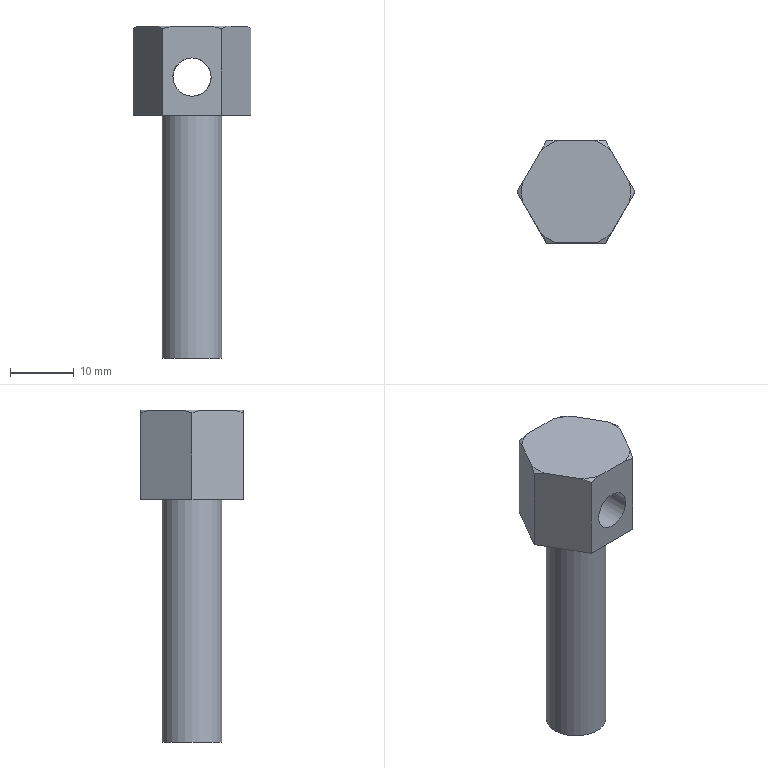Part | NX | features DATUM_CSYS 3, EXTRUDE 3, SKETCH 2, CHAMFER 1, CYLINDER 1, HOLE PACKAGE 1, SIMPLE HOLE 1, SYMBOLIC_THREAD 1 | 1 solid | 18 faces | box 18.475 x 16 x 52 mm | volume 4103 mm3 | plane 9 | cone 6 | cylinder 3 | commonest cylinder face diameters 6 x2 9.373 x1
STEP:
#1=CARTESIAN_POINT('',(4.619,8.,13.587));
#2=VERTEX_POINT('',#1);
#3=CARTESIAN_POINT('',(2.94,8.,14.));
#4=VERTEX_POINT('',#3);
#5=CARTESIAN_POINT('',(4.619,8.,13.587));
#6=CARTESIAN_POINT('',(4.067,8.,13.747));
#7=CARTESIAN_POINT('',(3.508,8.,13.887));
#8=CARTESIAN_POINT('',(2.94,8.,14.));
#9=B_SPLINE_CURVE_WITH_KNOTS('',3,(#5,#6,#7,#8),.UNSPECIFIED.,.F.,.F.,(4,4),(0.005943,0.007663),.UNSPECIFIED.);
#10=EDGE_CURVE('',#2,#4,#9,.T.);
#11=ORIENTED_EDGE('',*,*,#10,.F.);
#12=CARTESIAN_POINT('',(4.619,8.,0.));
#13=VERTEX_POINT('',#12);
#14=CARTESIAN_POINT('',(4.619,8.,14.));
#15=DIRECTION('',(0.,0.,-1.));
#16=VECTOR('',#15,1000.);
#17=LINE('',#14,#16);
#18=EDGE_CURVE('',#2,#13,#17,.T.);
#19=ORIENTED_EDGE('',*,*,#18,.T.);
#20=CARTESIAN_POINT('',(-4.619,8.,0.));
#21=VERTEX_POINT('',#20);
#22=CARTESIAN_POINT('',(-4.619,8.,0.));
#23=DIRECTION('',(1.,0.,0.));
#24=VECTOR('',#23,1000.);
#25=LINE('',#22,#24);
#26=EDGE_CURVE('',#21,#13,#25,.T.);
#27=ORIENTED_EDGE('',*,*,#26,.F.);
#28=CARTESIAN_POINT('',(-4.619,8.,13.587));
#29=VERTEX_POINT('',#28);
#30=CARTESIAN_POINT('',(-4.619,8.,14.));
#31=DIRECTION('',(0.,0.,-1.));
#32=VECTOR('',#31,1000.);
#33=LINE('',#30,#32);
#34=EDGE_CURVE('',#29,#21,#33,.T.);
#35=ORIENTED_EDGE('',*,*,#34,.F.);
#36=CARTESIAN_POINT('',(-2.94,8.,14.));
#37=VERTEX_POINT('',#36);
#38=CARTESIAN_POINT('',(-2.94,8.,14.));
#39=CARTESIAN_POINT('',(-3.508,8.,13.887));
#40=CARTESIAN_POINT('',(-4.067,8.,13.747));
#41=CARTESIAN_POINT('',(-4.619,8.,13.587));
#42=B_SPLINE_CURVE_WITH_KNOTS('',3,(#38,#39,#40,#41),.UNSPECIFIED.,.F.,.F.,(4,4),(0.01358,0.01531),.UNSPECIFIED.);
#43=EDGE_CURVE('',#37,#29,#42,.T.);
#44=ORIENTED_EDGE('',*,*,#43,.F.);
#45=CARTESIAN_POINT('',(-4.619,8.,14.));
#46=DIRECTION('',(1.,0.,0.));
#47=VECTOR('',#46,1000.);
#48=LINE('',#45,#47);
#49=EDGE_CURVE('',#37,#4,#48,.T.);
#50=ORIENTED_EDGE('',*,*,#49,.T.);
#51=EDGE_LOOP('',(#11,#19,#27,#35,#44,#50));
#52=FACE_BOUND('',#51,.T.);
#53=CARTESIAN_POINT('',(0.,8.,9.));
#54=VERTEX_POINT('',#53);
#55=CARTESIAN_POINT('',(0.,8.,6.));
#56=DIRECTION('',(0.,1.,0.));
#57=DIRECTION('',(0.,0.,1.));
#58=AXIS2_PLACEMENT_3D('',#55,#56,#57);
#59=CIRCLE('',#58,3.);
#60=EDGE_CURVE('',#54,#54,#59,.F.);
#61=ORIENTED_EDGE('',*,*,#60,.T.);
#62=EDGE_LOOP('',(#61));
#63=FACE_BOUND('',#62,.T.);
#64=CARTESIAN_POINT('',(-4.619,8.,14.));
#65=DIRECTION('',(0.,1.,0.));
#66=DIRECTION('',(0.,0.,1.));
#67=AXIS2_PLACEMENT_3D('',#64,#65,#66);
#68=PLANE('',#67);
#69=ADVANCED_FACE('',(#52,#63),#68,.T.);
#70=CARTESIAN_POINT('',(-4.619,-8.,13.587));
#71=VERTEX_POINT('',#70);
#72=CARTESIAN_POINT('',(-2.94,-8.,14.));
#73=VERTEX_POINT('',#72);
#74=CARTESIAN_POINT('',(-4.619,-8.,13.587));
#75=CARTESIAN_POINT('',(-4.067,-8.,13.747));
#76=CARTESIAN_POINT('',(-3.508,-8.,13.887));
#77=CARTESIAN_POINT('',(-2.94,-8.,14.));
#78=B_SPLINE_CURVE_WITH_KNOTS('',3,(#74,#75,#76,#77),.UNSPECIFIED.,.F.,.F.,(4,4),(0.005943,0.007663),.UNSPECIFIED.);
#79=EDGE_CURVE('',#71,#73,#78,.T.);
#80=ORIENTED_EDGE('',*,*,#79,.F.);
#81=CARTESIAN_POINT('',(-4.619,-8.,0.));
#82=VERTEX_POINT('',#81);
#83=CARTESIAN_POINT('',(-4.619,-8.,14.));
#84=DIRECTION('',(0.,0.,-1.));
#85=VECTOR('',#84,1000.);
#86=LINE('',#83,#85);
#87=EDGE_CURVE('',#71,#82,#86,.T.);
#88=ORIENTED_EDGE('',*,*,#87,.T.);
#89=CARTESIAN_POINT('',(4.619,-8.,0.));
#90=VERTEX_POINT('',#89);
#91=CARTESIAN_POINT('',(4.619,-8.,0.));
#92=DIRECTION('',(-1.,0.,0.));
#93=VECTOR('',#92,1000.);
#94=LINE('',#91,#93);
#95=EDGE_CURVE('',#90,#82,#94,.T.);
#96=ORIENTED_EDGE('',*,*,#95,.F.);
#97=CARTESIAN_POINT('',(4.619,-8.,13.587));
#98=VERTEX_POINT('',#97);
#99=CARTESIAN_POINT('',(4.619,-8.,14.));
#100=DIRECTION('',(0.,0.,-1.));
#101=VECTOR('',#100,1000.);
#102=LINE('',#99,#101);
#103=EDGE_CURVE('',#98,#90,#102,.T.);
#104=ORIENTED_EDGE('',*,*,#103,.F.);
#105=CARTESIAN_POINT('',(2.94,-8.,14.));
#106=VERTEX_POINT('',#105);
#107=CARTESIAN_POINT('',(2.94,-8.,14.));
#108=CARTESIAN_POINT('',(3.508,-8.,13.887));
#109=CARTESIAN_POINT('',(4.067,-8.,13.747));
#110=CARTESIAN_POINT('',(4.619,-8.,13.587));
#111=B_SPLINE_CURVE_WITH_KNOTS('',3,(#107,#108,#109,#110),.UNSPECIFIED.,.F.,.F.,(4,4),(0.01358,0.01531),.UNSPECIFIED.);
#112=EDGE_CURVE('',#106,#98,#111,.T.);
#113=ORIENTED_EDGE('',*,*,#112,.F.);
#114=CARTESIAN_POINT('',(4.619,-8.,14.));
#115=DIRECTION('',(-1.,0.,0.));
#116=VECTOR('',#115,1000.);
#117=LINE('',#114,#116);
#118=EDGE_CURVE('',#106,#73,#117,.T.);
#119=ORIENTED_EDGE('',*,*,#118,.T.);
#120=EDGE_LOOP('',(#80,#88,#96,#104,#113,#119));
#121=FACE_BOUND('',#120,.T.);
#122=CARTESIAN_POINT('',(3.,-8.,6.));
#123=VERTEX_POINT('',#122);
#124=CARTESIAN_POINT('',(0.,-8.,6.));
#125=DIRECTION('',(0.,-1.,0.));
#126=DIRECTION('',(1.,0.,0.));
#127=AXIS2_PLACEMENT_3D('',#124,#125,#126);
#128=CIRCLE('',#127,3.);
#129=EDGE_CURVE('',#123,#123,#128,.F.);
#130=ORIENTED_EDGE('',*,*,#129,.T.);
#131=EDGE_LOOP('',(#130));
#132=FACE_BOUND('',#131,.T.);
#133=CARTESIAN_POINT('',(4.619,-8.,14.));
#134=DIRECTION('',(0.,-1.,0.));
#135=DIRECTION('',(1.,0.,0.));
#136=AXIS2_PLACEMENT_3D('',#133,#134,#135);
#137=PLANE('',#136);
#138=ADVANCED_FACE('',(#121,#132),#137,.T.);
#139=CARTESIAN_POINT('',(3.,0.,-38.));
#140=VERTEX_POINT('',#139);
#141=CARTESIAN_POINT('',(0.,0.,-38.));
#142=DIRECTION('',(0.,0.,1.));
#143=DIRECTION('',(1.,0.,0.));
#144=AXIS2_PLACEMENT_3D('',#141,#142,#143);
#145=CIRCLE('',#144,3.);
#146=EDGE_CURVE('',#140,#140,#145,.T.);
#147=ORIENTED_EDGE('',*,*,#146,.F.);
#148=EDGE_LOOP('',(#147));
#149=FACE_BOUND('',#148,.T.);
#150=CARTESIAN_POINT('',(-3.,0.,6.));
#151=VERTEX_POINT('',#150);
#152=CARTESIAN_POINT('',(3.,0.,6.));
#153=VERTEX_POINT('',#152);
#154=CARTESIAN_POINT('',(0.,0.,6.));
#155=DIRECTION('',(0.,0.7071,0.7071));
#156=DIRECTION('',(0.,-0.7071,0.7071));
#157=AXIS2_PLACEMENT_3D('',#154,#155,#156);
#158=ELLIPSE('',#157,4.243,3.);
#159=EDGE_CURVE('',#151,#153,#158,.F.);
#160=ORIENTED_EDGE('',*,*,#159,.F.);
#161=CARTESIAN_POINT('',(0.,0.,6.));
#162=DIRECTION('',(0.,-0.7071,0.7071));
#163=DIRECTION('',(0.,0.7071,0.7071));
#164=AXIS2_PLACEMENT_3D('',#161,#162,#163);
#165=ELLIPSE('',#164,4.243,3.);
#166=EDGE_CURVE('',#153,#151,#165,.F.);
#167=ORIENTED_EDGE('',*,*,#166,.F.);
#168=EDGE_LOOP('',(#160,#167));
#169=FACE_BOUND('',#168,.T.);
#170=CARTESIAN_POINT('',(0.,0.,-38.));
#171=DIRECTION('',(0.,0.,1.));
#172=DIRECTION('',(1.,0.,0.));
#173=AXIS2_PLACEMENT_3D('',#170,#171,#172);
#174=CYLINDRICAL_SURFACE('',#173,3.);
#175=ADVANCED_FACE('',(#149,#169),#174,.F.);
#176=CARTESIAN_POINT('',(-8.398,1.454,14.));
#177=VERTEX_POINT('',#176);
#178=CARTESIAN_POINT('',(-9.238,0.,13.587));
#179=VERTEX_POINT('',#178);
#180=CARTESIAN_POINT('',(-8.398,1.454,14.));
#181=CARTESIAN_POINT('',(-8.682,0.963,13.887));
#182=CARTESIAN_POINT('',(-8.961,0.4789,13.747));
#183=CARTESIAN_POINT('',(-9.238,0.,13.587));
#184=B_SPLINE_CURVE_WITH_KNOTS('',3,(#180,#181,#182,#183),.UNSPECIFIED.,.F.,.F.,(4,4),(0.01453,0.01627),.UNSPECIFIED.);
#185=EDGE_CURVE('',#177,#179,#184,.T.);
#186=ORIENTED_EDGE('',*,*,#185,.T.);
#187=CARTESIAN_POINT('',(-8.398,-1.454,14.));
#188=VERTEX_POINT('',#187);
#189=CARTESIAN_POINT('',(-9.238,0.,13.587));
#190=CARTESIAN_POINT('',(-8.961,-0.479,13.747));
#191=CARTESIAN_POINT('',(-8.68,-0.9662,13.888));
#192=CARTESIAN_POINT('',(-8.398,-1.454,14.));
#193=B_SPLINE_CURVE_WITH_KNOTS('',3,(#189,#190,#191,#192),.UNSPECIFIED.,.F.,.F.,(4,4),(0.006888,0.008609),.UNSPECIFIED.);
#194=EDGE_CURVE('',#179,#188,#193,.T.);
#195=ORIENTED_EDGE('',*,*,#194,.T.);
#196=CARTESIAN_POINT('',(0.,0.,14.));
#197=DIRECTION('',(0.,0.,1.));
#198=DIRECTION('',(1.,0.,0.));
#199=AXIS2_PLACEMENT_3D('',#196,#197,#198);
#200=CIRCLE('',#199,8.523);
#201=EDGE_CURVE('',#177,#188,#200,.T.);
#202=ORIENTED_EDGE('',*,*,#201,.F.);
#203=EDGE_LOOP('',(#186,#195,#202));
#204=FACE_BOUND('',#203,.T.);
#205=CARTESIAN_POINT('',(0.,0.,14.));
#206=DIRECTION('',(0.,0.,-1.));
#207=DIRECTION('',(-1.,0.,0.));
#208=AXIS2_PLACEMENT_3D('',#205,#206,#207);
#209=CONICAL_SURFACE('',#208,8.523,1.047);
#210=ADVANCED_FACE('',(#204),#209,.T.);
#211=ORIENTED_EDGE('',*,*,#43,.T.);
#212=CARTESIAN_POINT('',(-5.458,6.546,14.));
#213=VERTEX_POINT('',#212);
#214=CARTESIAN_POINT('',(-4.619,8.,13.587));
#215=CARTESIAN_POINT('',(-4.895,7.521,13.747));
#216=CARTESIAN_POINT('',(-5.177,7.034,13.888));
#217=CARTESIAN_POINT('',(-5.458,6.546,14.));
#218=B_SPLINE_CURVE_WITH_KNOTS('',3,(#214,#215,#216,#217),.UNSPECIFIED.,.F.,.F.,(4,4),(0.006888,0.008609),.UNSPECIFIED.);
#219=EDGE_CURVE('',#29,#213,#218,.T.);
#220=ORIENTED_EDGE('',*,*,#219,.T.);
#221=CARTESIAN_POINT('',(0.,0.,14.));
#222=DIRECTION('',(0.,0.,1.));
#223=DIRECTION('',(1.,0.,0.));
#224=AXIS2_PLACEMENT_3D('',#221,#222,#223);
#225=CIRCLE('',#224,8.523);
#226=EDGE_CURVE('',#37,#213,#225,.T.);
#227=ORIENTED_EDGE('',*,*,#226,.F.);
#228=EDGE_LOOP('',(#211,#220,#227));
#229=FACE_BOUND('',#228,.T.);
#230=CARTESIAN_POINT('',(0.,0.,14.));
#231=DIRECTION('',(0.,0.,-1.));
#232=DIRECTION('',(-1.,0.,0.));
#233=AXIS2_PLACEMENT_3D('',#230,#231,#232);
#234=CONICAL_SURFACE('',#233,8.523,1.047);
#235=ADVANCED_FACE('',(#229),#234,.T.);
#236=CARTESIAN_POINT('',(5.458,6.546,14.));
#237=VERTEX_POINT('',#236);
#238=CARTESIAN_POINT('',(5.458,6.546,14.));
#239=CARTESIAN_POINT('',(5.175,7.037,13.887));
#240=CARTESIAN_POINT('',(4.895,7.521,13.747));
#241=CARTESIAN_POINT('',(4.619,8.,13.587));
#242=B_SPLINE_CURVE_WITH_KNOTS('',3,(#238,#239,#240,#241),.UNSPECIFIED.,.F.,.F.,(4,4),(0.01453,0.01627),.UNSPECIFIED.);
#243=EDGE_CURVE('',#237,#2,#242,.T.);
#244=ORIENTED_EDGE('',*,*,#243,.T.);
#245=ORIENTED_EDGE('',*,*,#10,.T.);
#246=CARTESIAN_POINT('',(0.,0.,14.));
#247=DIRECTION('',(0.,0.,1.));
#248=DIRECTION('',(1.,0.,0.));
#249=AXIS2_PLACEMENT_3D('',#246,#247,#248);
#250=CIRCLE('',#249,8.523);
#251=EDGE_CURVE('',#237,#4,#250,.T.);
#252=ORIENTED_EDGE('',*,*,#251,.F.);
#253=EDGE_LOOP('',(#244,#245,#252));
#254=FACE_BOUND('',#253,.T.);
#255=CARTESIAN_POINT('',(0.,0.,14.));
#256=DIRECTION('',(0.,0.,-1.));
#257=DIRECTION('',(-1.,0.,0.));
#258=AXIS2_PLACEMENT_3D('',#255,#256,#257);
#259=CONICAL_SURFACE('',#258,8.523,1.047);
#260=ADVANCED_FACE('',(#254),#259,.T.);
#261=CARTESIAN_POINT('',(8.398,-1.454,14.));
#262=VERTEX_POINT('',#261);
#263=CARTESIAN_POINT('',(9.238,0.,13.587));
#264=VERTEX_POINT('',#263);
#265=CARTESIAN_POINT('',(8.398,-1.454,14.));
#266=CARTESIAN_POINT('',(8.682,-0.963,13.887));
#267=CARTESIAN_POINT('',(8.961,-0.4789,13.747));
#268=CARTESIAN_POINT('',(9.238,0.,13.587));
#269=B_SPLINE_CURVE_WITH_KNOTS('',3,(#265,#266,#267,#268),.UNSPECIFIED.,.F.,.F.,(4,4),(0.01453,0.01627),.UNSPECIFIED.);
#270=EDGE_CURVE('',#262,#264,#269,.T.);
#271=ORIENTED_EDGE('',*,*,#270,.T.);
#272=CARTESIAN_POINT('',(8.398,1.454,14.));
#273=VERTEX_POINT('',#272);
#274=CARTESIAN_POINT('',(9.238,0.,13.587));
#275=CARTESIAN_POINT('',(8.961,0.479,13.747));
#276=CARTESIAN_POINT('',(8.68,0.9662,13.888));
#277=CARTESIAN_POINT('',(8.398,1.454,14.));
#278=B_SPLINE_CURVE_WITH_KNOTS('',3,(#274,#275,#276,#277),.UNSPECIFIED.,.F.,.F.,(4,4),(0.006888,0.008609),.UNSPECIFIED.);
#279=EDGE_CURVE('',#264,#273,#278,.T.);
#280=ORIENTED_EDGE('',*,*,#279,.T.);
#281=CARTESIAN_POINT('',(0.,0.,14.));
#282=DIRECTION('',(0.,0.,1.));
#283=DIRECTION('',(1.,0.,0.));
#284=AXIS2_PLACEMENT_3D('',#281,#282,#283);
#285=CIRCLE('',#284,8.523);
#286=EDGE_CURVE('',#262,#273,#285,.T.);
#287=ORIENTED_EDGE('',*,*,#286,.F.);
#288=EDGE_LOOP('',(#271,#280,#287));
#289=FACE_BOUND('',#288,.T.);
#290=CARTESIAN_POINT('',(0.,0.,14.));
#291=DIRECTION('',(0.,0.,-1.));
#292=DIRECTION('',(-1.,0.,0.));
#293=AXIS2_PLACEMENT_3D('',#290,#291,#292);
#294=CONICAL_SURFACE('',#293,8.523,1.047);
#295=ADVANCED_FACE('',(#289),#294,.T.);
#296=ORIENTED_EDGE('',*,*,#112,.T.);
#297=CARTESIAN_POINT('',(5.458,-6.546,14.));
#298=VERTEX_POINT('',#297);
#299=CARTESIAN_POINT('',(4.619,-8.,13.587));
#300=CARTESIAN_POINT('',(4.895,-7.521,13.747));
#301=CARTESIAN_POINT('',(5.177,-7.034,13.888));
#302=CARTESIAN_POINT('',(5.458,-6.546,14.));
#303=B_SPLINE_CURVE_WITH_KNOTS('',3,(#299,#300,#301,#302),.UNSPECIFIED.,.F.,.F.,(4,4),(0.006888,0.008609),.UNSPECIFIED.);
#304=EDGE_CURVE('',#98,#298,#303,.T.);
#305=ORIENTED_EDGE('',*,*,#304,.T.);
#306=CARTESIAN_POINT('',(0.,0.,14.));
#307=DIRECTION('',(0.,0.,1.));
#308=DIRECTION('',(1.,0.,0.));
#309=AXIS2_PLACEMENT_3D('',#306,#307,#308);
#310=CIRCLE('',#309,8.523);
#311=EDGE_CURVE('',#106,#298,#310,.T.);
#312=ORIENTED_EDGE('',*,*,#311,.F.);
#313=EDGE_LOOP('',(#296,#305,#312));
#314=FACE_BOUND('',#313,.T.);
#315=CARTESIAN_POINT('',(0.,0.,14.));
#316=DIRECTION('',(0.,0.,-1.));
#317=DIRECTION('',(-1.,0.,0.));
#318=AXIS2_PLACEMENT_3D('',#315,#316,#317);
#319=CONICAL_SURFACE('',#318,8.523,1.047);
#320=ADVANCED_FACE('',(#314),#319,.T.);
#321=CARTESIAN_POINT('',(-5.458,-6.546,14.));
#322=VERTEX_POINT('',#321);
#323=CARTESIAN_POINT('',(0.,0.,14.));
#324=DIRECTION('',(0.,0.,1.));
#325=DIRECTION('',(1.,0.,0.));
#326=AXIS2_PLACEMENT_3D('',#323,#324,#325);
#327=CIRCLE('',#326,8.523);
#328=EDGE_CURVE('',#322,#73,#327,.T.);
#329=ORIENTED_EDGE('',*,*,#328,.F.);
#330=CARTESIAN_POINT('',(-5.458,-6.546,14.));
#331=CARTESIAN_POINT('',(-5.175,-7.037,13.887));
#332=CARTESIAN_POINT('',(-4.895,-7.521,13.747));
#333=CARTESIAN_POINT('',(-4.619,-8.,13.587));
#334=B_SPLINE_CURVE_WITH_KNOTS('',3,(#330,#331,#332,#333),.UNSPECIFIED.,.F.,.F.,(4,4),(0.01453,0.01627),.UNSPECIFIED.);
#335=EDGE_CURVE('',#322,#71,#334,.T.);
#336=ORIENTED_EDGE('',*,*,#335,.T.);
#337=ORIENTED_EDGE('',*,*,#79,.T.);
#338=EDGE_LOOP('',(#329,#336,#337));
#339=FACE_BOUND('',#338,.T.);
#340=CARTESIAN_POINT('',(0.,0.,14.));
#341=DIRECTION('',(0.,0.,-1.));
#342=DIRECTION('',(-1.,0.,0.));
#343=AXIS2_PLACEMENT_3D('',#340,#341,#342);
#344=CONICAL_SURFACE('',#343,8.523,1.047);
#345=ADVANCED_FACE('',(#339),#344,.T.);
#346=CARTESIAN_POINT('',(-4.619,-8.,14.));
#347=DIRECTION('',(-0.5,0.866,0.));
#348=VECTOR('',#347,1000.);
#349=LINE('',#346,#348);
#350=EDGE_CURVE('',#322,#188,#349,.T.);
#351=ORIENTED_EDGE('',*,*,#350,.F.);
#352=ORIENTED_EDGE('',*,*,#328,.T.);
#353=ORIENTED_EDGE('',*,*,#118,.F.);
#354=ORIENTED_EDGE('',*,*,#311,.T.);
#355=CARTESIAN_POINT('',(9.238,0.,14.));
#356=DIRECTION('',(-0.5,-0.866,0.));
#357=VECTOR('',#356,1000.);
#358=LINE('',#355,#357);
#359=EDGE_CURVE('',#262,#298,#358,.T.);
#360=ORIENTED_EDGE('',*,*,#359,.F.);
#361=ORIENTED_EDGE('',*,*,#286,.T.);
#362=CARTESIAN_POINT('',(4.619,8.,14.));
#363=DIRECTION('',(0.5,-0.866,0.));
#364=VECTOR('',#363,1000.);
#365=LINE('',#362,#364);
#366=EDGE_CURVE('',#237,#273,#365,.T.);
#367=ORIENTED_EDGE('',*,*,#366,.F.);
#368=ORIENTED_EDGE('',*,*,#251,.T.);
#369=ORIENTED_EDGE('',*,*,#49,.F.);
#370=ORIENTED_EDGE('',*,*,#226,.T.);
#371=CARTESIAN_POINT('',(-9.238,0.,14.));
#372=DIRECTION('',(0.5,0.866,0.));
#373=VECTOR('',#372,1000.);
#374=LINE('',#371,#373);
#375=EDGE_CURVE('',#177,#213,#374,.T.);
#376=ORIENTED_EDGE('',*,*,#375,.F.);
#377=ORIENTED_EDGE('',*,*,#201,.T.);
#378=EDGE_LOOP('',(#351,#352,#353,#354,#360,#361,#367,#368,#369,#370,#376,#377));
#379=FACE_BOUND('',#378,.T.);
#380=CARTESIAN_POINT('',(0.,0.,14.));
#381=DIRECTION('',(0.,0.,1.));
#382=DIRECTION('',(1.,0.,0.));
#383=AXIS2_PLACEMENT_3D('',#380,#381,#382);
#384=PLANE('',#383);
#385=ADVANCED_FACE('',(#379),#384,.T.);
#386=ORIENTED_EDGE('',*,*,#194,.F.);
#387=CARTESIAN_POINT('',(-9.238,0.,0.));
#388=VERTEX_POINT('',#387);
#389=CARTESIAN_POINT('',(-9.238,0.,14.));
#390=DIRECTION('',(0.,0.,-1.));
#391=VECTOR('',#390,1000.);
#392=LINE('',#389,#391);
#393=EDGE_CURVE('',#179,#388,#392,.T.);
#394=ORIENTED_EDGE('',*,*,#393,.T.);
#395=CARTESIAN_POINT('',(-4.619,-8.,0.));
#396=DIRECTION('',(-0.5,0.866,0.));
#397=VECTOR('',#396,1000.);
#398=LINE('',#395,#397);
#399=EDGE_CURVE('',#82,#388,#398,.T.);
#400=ORIENTED_EDGE('',*,*,#399,.F.);
#401=ORIENTED_EDGE('',*,*,#87,.F.);
#402=ORIENTED_EDGE('',*,*,#335,.F.);
#403=ORIENTED_EDGE('',*,*,#350,.T.);
#404=EDGE_LOOP('',(#386,#394,#400,#401,#402,#403));
#405=FACE_BOUND('',#404,.T.);
#406=CARTESIAN_POINT('',(-4.619,-8.,14.));
#407=DIRECTION('',(-0.866,-0.5,0.));
#408=DIRECTION('',(0.5,-0.866,0.));
#409=AXIS2_PLACEMENT_3D('',#406,#407,#408);
#410=PLANE('',#409);
#411=ADVANCED_FACE('',(#405),#410,.T.);
#412=ORIENTED_EDGE('',*,*,#219,.F.);
#413=ORIENTED_EDGE('',*,*,#34,.T.);
#414=CARTESIAN_POINT('',(-9.238,0.,0.));
#415=DIRECTION('',(0.5,0.866,0.));
#416=VECTOR('',#415,1000.);
#417=LINE('',#414,#416);
#418=EDGE_CURVE('',#388,#21,#417,.T.);
#419=ORIENTED_EDGE('',*,*,#418,.F.);
#420=ORIENTED_EDGE('',*,*,#393,.F.);
#421=ORIENTED_EDGE('',*,*,#185,.F.);
#422=ORIENTED_EDGE('',*,*,#375,.T.);
#423=EDGE_LOOP('',(#412,#413,#419,#420,#421,#422));
#424=FACE_BOUND('',#423,.T.);
#425=CARTESIAN_POINT('',(-9.238,0.,14.));
#426=DIRECTION('',(-0.866,0.5,0.));
#427=DIRECTION('',(-0.5,-0.866,0.));
#428=AXIS2_PLACEMENT_3D('',#425,#426,#427);
#429=PLANE('',#428);
#430=ADVANCED_FACE('',(#424),#429,.T.);
#431=ORIENTED_EDGE('',*,*,#279,.F.);
#432=CARTESIAN_POINT('',(9.238,0.,0.));
#433=VERTEX_POINT('',#432);
#434=CARTESIAN_POINT('',(9.238,0.,14.));
#435=DIRECTION('',(0.,0.,-1.));
#436=VECTOR('',#435,1000.);
#437=LINE('',#434,#436);
#438=EDGE_CURVE('',#264,#433,#437,.T.);
#439=ORIENTED_EDGE('',*,*,#438,.T.);
#440=CARTESIAN_POINT('',(4.619,8.,0.));
#441=DIRECTION('',(0.5,-0.866,0.));
#442=VECTOR('',#441,1000.);
#443=LINE('',#440,#442);
#444=EDGE_CURVE('',#13,#433,#443,.T.);
#445=ORIENTED_EDGE('',*,*,#444,.F.);
#446=ORIENTED_EDGE('',*,*,#18,.F.);
#447=ORIENTED_EDGE('',*,*,#243,.F.);
#448=ORIENTED_EDGE('',*,*,#366,.T.);
#449=EDGE_LOOP('',(#431,#439,#445,#446,#447,#448));
#450=FACE_BOUND('',#449,.T.);
#451=CARTESIAN_POINT('',(4.619,8.,14.));
#452=DIRECTION('',(0.866,0.5,0.));
#453=DIRECTION('',(-0.5,0.866,0.));
#454=AXIS2_PLACEMENT_3D('',#451,#452,#453);
#455=PLANE('',#454);
#456=ADVANCED_FACE('',(#450),#455,.T.);
#457=ORIENTED_EDGE('',*,*,#304,.F.);
#458=ORIENTED_EDGE('',*,*,#103,.T.);
#459=CARTESIAN_POINT('',(9.238,0.,0.));
#460=DIRECTION('',(-0.5,-0.866,0.));
#461=VECTOR('',#460,1000.);
#462=LINE('',#459,#461);
#463=EDGE_CURVE('',#433,#90,#462,.T.);
#464=ORIENTED_EDGE('',*,*,#463,.F.);
#465=ORIENTED_EDGE('',*,*,#438,.F.);
#466=ORIENTED_EDGE('',*,*,#270,.F.);
#467=ORIENTED_EDGE('',*,*,#359,.T.);
#468=EDGE_LOOP('',(#457,#458,#464,#465,#466,#467));
#469=FACE_BOUND('',#468,.T.);
#470=CARTESIAN_POINT('',(9.238,0.,14.));
#471=DIRECTION('',(0.866,-0.5,0.));
#472=DIRECTION('',(0.5,0.866,0.));
#473=AXIS2_PLACEMENT_3D('',#470,#471,#472);
#474=PLANE('',#473);
#475=ADVANCED_FACE('',(#469),#474,.T.);
#476=CARTESIAN_POINT('',(-4.686,0.,0.));
#477=VERTEX_POINT('',#476);
#478=CARTESIAN_POINT('',(0.,0.,0.));
#479=DIRECTION('',(0.,0.,-1.));
#480=DIRECTION('',(-1.,0.,0.));
#481=AXIS2_PLACEMENT_3D('',#478,#479,#480);
#482=CIRCLE('',#481,4.686);
#483=EDGE_CURVE('',#477,#477,#482,.T.);
#484=ORIENTED_EDGE('',*,*,#483,.F.);
#485=EDGE_LOOP('',(#484));
#486=FACE_BOUND('',#485,.T.);
#487=ORIENTED_EDGE('',*,*,#95,.T.);
#488=ORIENTED_EDGE('',*,*,#399,.T.);
#489=ORIENTED_EDGE('',*,*,#418,.T.);
#490=ORIENTED_EDGE('',*,*,#26,.T.);
#491=ORIENTED_EDGE('',*,*,#444,.T.);
#492=ORIENTED_EDGE('',*,*,#463,.T.);
#493=EDGE_LOOP('',(#487,#488,#489,#490,#491,#492));
#494=FACE_BOUND('',#493,.T.);
#495=CARTESIAN_POINT('',(0.,0.,0.));
#496=DIRECTION('',(0.,0.,1.));
#497=DIRECTION('',(1.,0.,0.));
#498=AXIS2_PLACEMENT_3D('',#495,#496,#497);
#499=PLANE('',#498);
#500=ADVANCED_FACE('',(#486,#494),#499,.F.);
#501=ORIENTED_EDGE('',*,*,#146,.T.);
#502=EDGE_LOOP('',(#501));
#503=FACE_BOUND('',#502,.T.);
#504=CARTESIAN_POINT('',(4.686,0.,-38.));
#505=VERTEX_POINT('',#504);
#506=CARTESIAN_POINT('',(0.,0.,-38.));
#507=DIRECTION('',(0.,0.,1.));
#508=DIRECTION('',(1.,0.,0.));
#509=AXIS2_PLACEMENT_3D('',#506,#507,#508);
#510=CIRCLE('',#509,4.686);
#511=EDGE_CURVE('',#505,#505,#510,.T.);
#512=ORIENTED_EDGE('',*,*,#511,.F.);
#513=EDGE_LOOP('',(#512));
#514=FACE_BOUND('',#513,.T.);
#515=CARTESIAN_POINT('',(0.,0.,-38.));
#516=DIRECTION('',(0.,0.,-1.));
#517=DIRECTION('',(-1.,0.,0.));
#518=AXIS2_PLACEMENT_3D('',#515,#516,#517);
#519=PLANE('',#518);
#520=ADVANCED_FACE('',(#503,#514),#519,.T.);
#521=ORIENTED_EDGE('',*,*,#511,.T.);
#522=EDGE_LOOP('',(#521));
#523=FACE_BOUND('',#522,.T.);
#524=ORIENTED_EDGE('',*,*,#483,.T.);
#525=EDGE_LOOP('',(#524));
#526=FACE_BOUND('',#525,.T.);
#527=CARTESIAN_POINT('',(0.,0.,0.));
#528=DIRECTION('',(0.,0.,-1.));
#529=DIRECTION('',(-1.,0.,0.));
#530=AXIS2_PLACEMENT_3D('',#527,#528,#529);
#531=CYLINDRICAL_SURFACE('',#530,4.686);
#532=ADVANCED_FACE('',(#523,#526),#531,.T.);
#533=ORIENTED_EDGE('',*,*,#60,.F.);
#534=EDGE_LOOP('',(#533));
#535=FACE_BOUND('',#534,.T.);
#536=ORIENTED_EDGE('',*,*,#129,.F.);
#537=EDGE_LOOP('',(#536));
#538=FACE_BOUND('',#537,.T.);
#539=ORIENTED_EDGE('',*,*,#159,.T.);
#540=ORIENTED_EDGE('',*,*,#166,.T.);
#541=EDGE_LOOP('',(#539,#540));
#542=FACE_BOUND('',#541,.T.);
#543=CARTESIAN_POINT('',(0.,-14.,6.));
#544=DIRECTION('',(0.,1.,0.));
#545=DIRECTION('',(0.,0.,1.));
#546=AXIS2_PLACEMENT_3D('',#543,#544,#545);
#547=CYLINDRICAL_SURFACE('',#546,3.);
#548=ADVANCED_FACE('',(#535,#538,#542),#547,.F.);
#549=CLOSED_SHELL('',(#69,#138,#175,#210,#235,#260,#295,#320,#345,#385,#411,#430,#456,#475,#500,#520,#532,#548));
#550=MANIFOLD_SOLID_BREP('',#549);
#551=(LENGTH_UNIT()NAMED_UNIT(*)SI_UNIT(.MILLI.,.METRE.));
#552=UNCERTAINTY_MEASURE_WITH_UNIT(LENGTH_MEASURE(0.0508),#551,'','');
#553=(NAMED_UNIT(*)PLANE_ANGLE_UNIT()SI_UNIT($,.RADIAN.));
#554=(NAMED_UNIT(*)SI_UNIT($,.STERADIAN.)SOLID_ANGLE_UNIT());
#555=(GEOMETRIC_REPRESENTATION_CONTEXT(3)GLOBAL_UNCERTAINTY_ASSIGNED_CONTEXT((#552))GLOBAL_UNIT_ASSIGNED_CONTEXT((#551,#553,#554))REPRESENTATION_CONTEXT('',''));
#556=ADVANCED_BREP_SHAPE_REPRESENTATION('',(#550),#555);